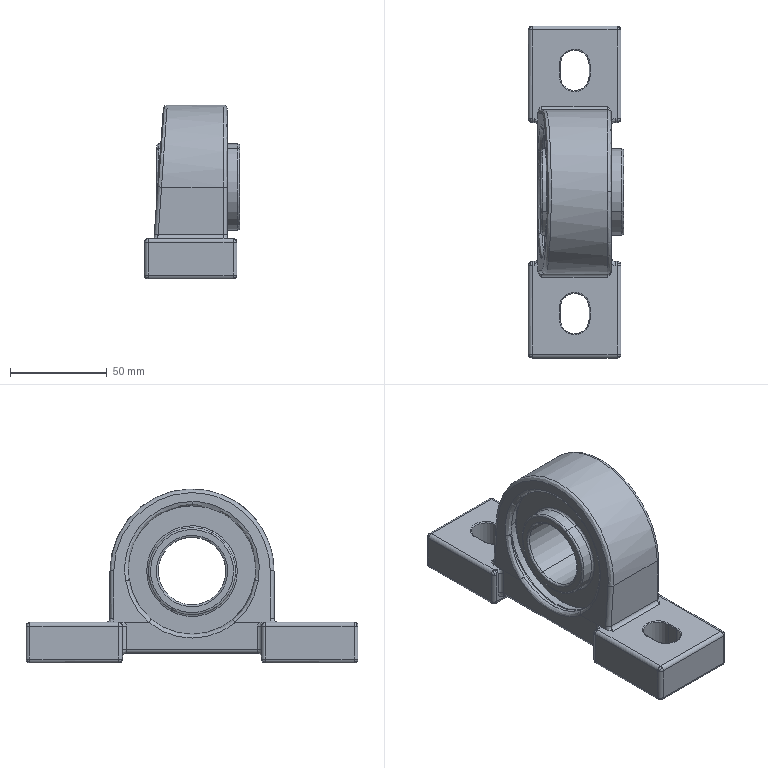Part | SolidWorks | features LayoutProfileFeature 1 | 2 solids | 175 faces | box 49.4 x 172 x 90.1 mm | volume 253379 mm3 | spline 86 | cylinder 63 | plane 26 | commonest cylinder face diameters 4 x40 1 x8 15 x4 45 x4 65.452 x4 35 x2